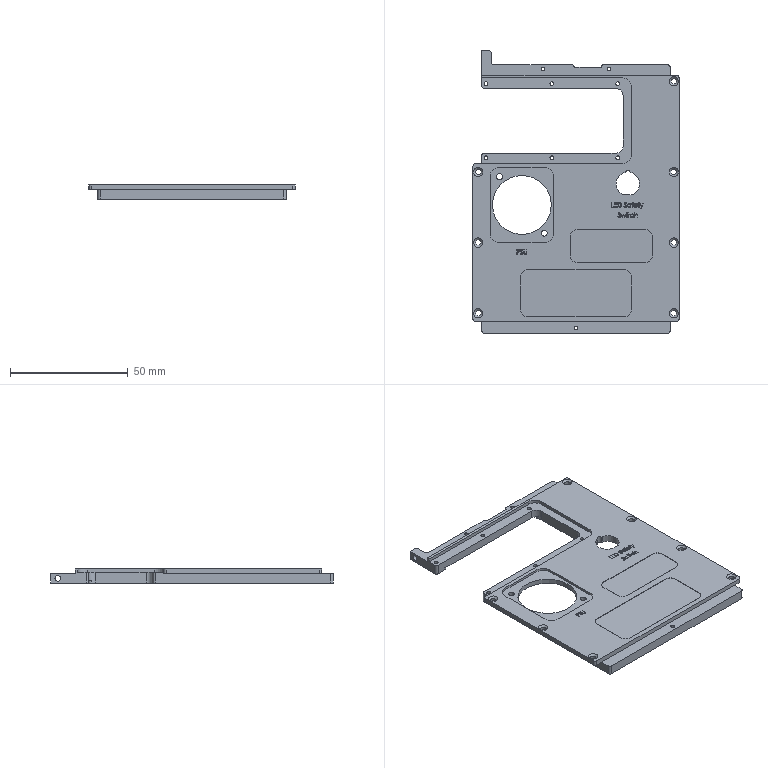NC program | NX | posted with a generic post | part box 87.5 x 120 x 6.001 mm
Whole program:
N10 G17 G21 G94 G90
(FLOOR_WALL_2 , TOOL : D63面刀)
N12 T01 M6
N14 G54
N16 G17 G0 G90 X96. Y-5. B0. C0. S4000 M3
N18 G43 Z50.001 H1
N20 Z6.545
N22 G94 G1 Z3.545 F1500.
N24 X86.
N26 X-97.
N28 Y41.55
N30 X86.
N32 X96.
N34 Z6.545
N36 G0 Z50.001
N38 Y-5.
N40 Z6.089
N42 G1 Z3.089
N44 X86.
N46 X-97.
N48 Y41.55
N50 X86.
N52 X96.
N54 Z6.089
N56 G0 Z50.001
N58 Y-5.
N60 Z5.632
N62 G1 Z2.632
N64 X86.
N66 X-97.
N68 Y41.55
N70 X86.
N72 X96.
N74 Z5.632
N76 G0 Z50.001
N78 Y-5.
N80 Z5.176
N82 G1 Z2.176
N84 X86.
N86 X-97.
N88 Y41.55
N90 X86.
N92 X96.
N94 Z5.176
N96 G0 Z50.001
N98 Y-5.
N100 Z4.72
N102 G1 Z1.72
N104 X86.
N106 X-97.
N108 Y41.55
N110 X86.
N112 X96.
N114 Z4.72
N116 G0 Z50.001
N118 Y-5.
N120 Z4.264
N122 G1 Z1.264
N124 X86.
N126 X-97.
N128 Y41.55
N130 X86.
N132 X96.
N134 Z4.264
N136 G0 Z50.001
N138 Y-5.
N140 Z3.807
N142 G1 Z0.807
N144 X86.
N146 X-97.
N148 Y41.55
N150 X86.
N152 X96.
N154 Z3.807
N156 G0 Z50.001
N158 Y-5.
N160 Z3.351
N162 G1 Z0.351
N164 X86.
N166 X-97.
N168 Y41.55
N170 X86.
N172 X96.
N174 Z3.351
N176 G0 Z50.001
N178 M5
(FLOOR_WALL_2_COPY , TOOL : D12-35-D12-75波刀)
N180 T13 M6
N182 G54
N184 G17 G0 G90 X70.5 Y-17.75 B0. C0. S4000 M3
N186 G43 Z50.001 H13
N188 Z3.031
N190 G94 G1 Z0.031 F1500.
N192 X60.5
N194 X-71.5
N196 Y-8.894
N198 X60.5
N200 Y-0.039
N202 X-71.5
N204 Y8.817
N206 X60.5
N208 Y17.672
N210 X-71.5
N212 Y26.528
N214 X60.5
N216 Y35.383
N218 X-71.5
N220 Y44.239
N222 X60.5
N224 Y53.094
N226 X-71.5
N228 Y61.95
N230 X60.5
N232 X70.5
N234 Z3.031
N236 G0 Z50.001
(FLOOR_WALL_2_COPY_COPY , TOOL : D12-35-D12-75波刀)
N238 Y-17.75 S5000
N240 Z3.001
N242 G1 Z0.001 F500.
N244 X60.5
N246 X-71.5
N248 Y-8.894
N250 X60.5
N252 Y-0.039
N254 X-71.5
N256 Y8.817
N258 X60.5
N260 Y17.672
N262 X-71.5
N264 Y26.528
N266 X60.5
N268 Y35.383
N270 X-71.5
N272 Y44.239
N274 X60.5
N276 Y53.094
N278 X-71.5
N280 Y61.95
N282 X60.5
N284 X70.5
N286 Z3.001
N288 G0 Z50.001
N290 M5
(PLANAR_MILL_5 , TOOL : D6-18-D6-50-3T-ROUGH)
N292 T02 M6
N294 G54
N296 G17 G0 G90 X0. Y-4.4 B0. C0. S5500 M3
N298 G43 Z50.001 H2
N300 Z2.5
N302 G94 G1 Z-0.5 F2500.
N304 Y-7.4
N306 X9.9
N308 Y7.4
N310 X-9.9
N312 Y-7.4
N314 X0.
N316 Y-4.4
N318 Y-10.4
N320 X12.
N322 G3 X12.9 Y-9.5 R0.9
N324 G1 Y9.5
N326 G3 X12. Y10.4 R0.9
N328 G1 X-12.
N330 G3 X-12.9 Y9.5 R0.9
N332 G1 Y-9.5
N334 G3 X-12. Y-10.4 R0.9
N336 G1 X0.
N338 Y-7.4
N340 Z2.5
N342 G0 Z50.001
N344 Y-4.4
N346 Z2.1
N348 G1 Z-0.9
N350 Y-7.4
N352 X9.9
N354 Y7.4
N356 X-9.9
N358 Y-7.4
N360 X0.
N362 Y-4.4
N364 Y-10.4
N366 X12.
N368 G3 X12.9 Y-9.5 R0.9
N370 G1 Y9.5
N372 G3 X12. Y10.4 R0.9
N374 G1 X-12.
N376 G3 X-12.9 Y9.5 R0.9
N378 G1 Y-9.5
N380 G3 X-12. Y-10.4 R0.9
N382 G1 X0.
N384 Y-7.4
N386 Z2.1
N388 G0 Z50.001
(PLANAR_MILL_5_COPY_2 , TOOL : D6-18-D6-50-3T-ROUGH)
N390 X-20.6 Y-25.75
N392 Z2.5
N394 G1 Z-0.5
N396 Y-19.75
N398 Y42.5
N400 G3 X-21.5 Y43.4 R0.9
N402 G1 X-50.
N404 G3 X-50.9 Y42.5 R0.9
N406 G1 Y-17.
N408 Y-23.
N410 Z2.5
N412 G0 X-20.6 Y-25.75 Z2.
N414 G1 Z-1.
N416 Y-19.75
N418 Y42.5
N420 G3 X-21.5 Y43.4 R0.9
N422 G1 X-50.
N424 G3 X-50.9 Y42.5 R0.9
N426 G1 Y-17.
N428 Y-23.
N430 Z2.
N432 G0 X-20.6 Y-25.75 Z1.6
N434 G1 Z-1.4
N436 Y-19.75
N438 Y42.5
N440 G3 X-21.5 Y43.4 R0.9
N442 G1 X-50.
N444 G3 X-50.9 Y42.5 R0.9
N446 G1 Y-17.
N448 Y-23.
N450 Z1.6
N452 G0 Z50.001
N454 M5
(PLANAR_MILL_5_COPY , TOOL : D6-18-D6-50-3T-FINISH)
N456 T05 M6
N458 G54
N460 G17 G0 G90 X17.458 Y49. B0. C0. S5464 M3
N462 G43 Z50.001 H5
N464 Z0.
N466 G94 G1 X17. Z-0.008 F500.
N468 Y38. Z-0.2
N470 X16.5
N472 Y26.5
N474 X18.5
N476 Y49.5
N478 X16.5
N480 Y38.
N482 Z0.
N484 G0 X14. Y49.458
N486 G1 Y38. Z-0.2
N488 X13.5
N490 Y23.5
N492 X21.5
N494 Y52.5
N496 X13.5
N498 Y38.
N500 X14.025 Z0.325
N502 G0 Z50.001
N504 X39.8 Y11.542
N506 Z0.
N508 G1 Y23. Z-0.2
N510 X40.3
N512 Y39.3
N514 X34.7
N516 Y6.7
N518 X40.3
N520 Y23.
N522 Z0.
N524 G0 X44. Y11.542
N526 G1 Y23. Z-0.2
N528 X44.5
N530 Y43.5
N532 X30.5
N534 Y2.5
N536 X44.5
N538 Y23.
N540 X43.975 Z0.325
N542 G0 Z50.001
(PLANAR_MILL_5_COPY_1 , TOOL : D6-18-D6-50-3T-FINISH)
N544 X-0.5 Y-7.
N546 Z2.
N548 G1 Z-1.
N550 G3 X0. Y-7.5 R0.5
N552 G1 X10.
N554 Y7.5
N556 X-10.
N558 Y-7.5
N560 X0.
N562 G3 X0.5 Y-7. R0.5
N564 G1 X-0.5 Y-10.
N566 G3 X0. Y-10.5 R0.5
N568 G1 X12.
N570 G3 X13. Y-9.5 R1.
N572 G1 Y9.5
N574 G3 X12. Y10.5 R1.
N576 G1 X-12.
N578 G3 X-13. Y9.5 R1.
N580 G1 Y-9.5
N582 G3 X-12. Y-10.5 R1.
N584 G1 X0.
N586 G3 X0.5 Y-10. R0.5
N588 G1 Z2.
N590 G0 Z50.001
(PLANAR_MILL_5_COPY_2_COPY , TOOL : D6-18-D6-50-3T-FINISH)
N592 X-20.5 Y-25.75
N594 Z1.5
N596 G1 Z-1.5
N598 Y-19.75
N600 Y42.5
N602 G3 X-21.5 Y43.5 R1.
N604 G1 X-50.
N606 G3 X-51. Y42.5 R1.
N608 G1 Y-17.
N610 Y-23.
N612 Z1.5
N614 G0 Z50.001
N616 M5
(PLANAR_MILL_4 , TOOL : D12-35-D12-75波刀)
N618 T13 M6
N620 G54
N622 G17 G0 G90 X55.6 Y77.75 B0. C0. S5500 M3
N624 G43 Z50.001 H13
N626 Z2.
N628 G94 G1 Z-1. F2500.
N630 Y65.75
N632 Y-19.75
N634 Y-31.75
N636 Z2.
N638 G0 Z3.
N640 Y77.75
N642 Z1.1
N644 G1 Z-1.9
N646 Y65.75
N648 Y-19.75
N650 Y-31.75
N652 Z1.1
N654 G0 Z50.001
(PLANAR_MILL_4_COPY , TOOL : D12-35-D12-75波刀)
N656 X-61.1 Y-29.
N658 Z2.
N660 G1 Z-1.
N662 Y-17.
N664 Y65.75
N666 Y77.75
N668 Z2.
N670 G0 Z3.
N672 Y-29.
N674 Z1.1
N676 G1 Z-1.9
N678 Y-17.
N680 Y65.75
N682 Y77.75
N684 Z1.1
N686 G0 Z50.001
N688 M5
(PLANAR_MILL_4_COPY_COPY , TOOL : D6-18-D6-50-3T-FINISH)
N690 T05 M6
N692 G54
N694 G17 G0 G90 X-63.5 Y-8. B0. C0. S5500 M3
N696 G43 Z50.001 H5
N698 Z1.
N700 G94 G1 Z-2. F2500.
N702 Y-14.
N704 Y-17.
N706 Y-23.
N708 Z1.
N710 G0 Z50.001
(PLANAR_MILL_4_COPY_COPY_COPY , TOOL : D6-18-D6-50-3T-FINISH)
N712 X-59. Y-18.
N714 Z1.
N716 G1 Z-2.
N718 G3 X-58. Y-17. R1.
N720 G1 Y65.75
N722 G2 X-54. Y69.75 R4.
N724 G1 X48.5
N726 G2 X52.5 Y65.75 R4.
N728 G1 Y-19.75
N730 G2 X48.5 Y-23.75 R4.
N732 G1 X-16.5
N734 G3 X-17.5 Y-24.75 R1.
N736 G1 Z1.
N738 G0 Z50.001
N740 M5
(SPOT_DRILLING_2 , TOOL : 点孔D5-120-90度)
N742 T14 M6
N744 G54
N746 G17 G0 G90 X-14. Y-18.5 B0. C0. S2500 M3
N748 G43 Z50.001 H14
N750 G94 G82 G99 Z-2. F120. P200 R2.
N752 X16.
N754 X46.
N756 Y64.5
N758 X16.
N760 X-14.
N762 X-52.5
N764 G80
N766 G0 X-52.5 Y64.5 Z50.001
(SPOT_DRILLING_2_COPY , TOOL : 点孔D5-120-90度)
N768 X-12. Y-9.5
N770 G82 Z-2.25 F120. P200 R1.
N772 X12. Y9.5
N774 G80
N776 G0 X12. Y9.5 Z50.001
N778 M5
(SPOT_DRILLING_2_COPY_COPY , TOOL : 点孔D3-50-90度)
N780 T07 M6
N782 G54
N784 G17 G0 G90 X52.25 Y23. B0. C0. S2500 M3
N786 G43 Z10. H7
N788 G94 G82 G98 Z-3.02 F120. P200 R0.
N790 X-20. Y40.75 Z-2.52 R0.5
N792 Y12.75
N794 Y-15.25
N796 X-51.5
N798 X-57.75 Y9. Z-3.02 R0.
N800 X-51.5 Y12.75 Z-2.52 R0.5
N802 X-57.75 Y37. Z-3.02 R0.
N804 X-51.5 Y40.75 Z-2.52 R0.5
N806 G80
N808 G0 X-51.5 Y40.75 Z10.
(PLANAR_MILL_7 , TOOL : 点孔D3-50-90度)
N810 Z50.001 S6500
N812 X-2.75 Y69.05
N814 Z2.2
N816 G1 Z-0.8 F1500.
N818 Y67.55
N820 X48.5
N822 G2 X50.3 Y65.75 R1.8
N824 G1 Y-19.75
N826 G2 X48.5 Y-21.55 R1.8
N828 G1 X-16.5
N830 G2 X-18.3 Y-19.75 R1.8
N832 G1 Y42.5
N834 G3 X-21.5 Y45.7 R3.2
N836 G1 X-50.
N838 G3 X-53.2 Y42.5 R3.2
N840 G1 Y-17.
N842 G2 X-54. Y-17.8 R0.8
N844 G1 X-55.
N846 G2 X-55.8 Y-17. R0.8
N848 G1 Y65.75
N850 G2 X-54. Y67.55 R1.8
N852 G1 X-2.75
N854 Y69.05
N856 Z2.2
N858 G0 Z50.001
(PLANAR_MILL_7_COPY_1 , TOOL : 点孔D3-50-90度)
N860 X-20.5 Y-18.3
N862 Z0.7
N864 G1 Z-2.3
N866 G3 X-21. Y-17.8 R0.5
N868 G2 X-22.8 Y-16. R1.8
N870 G1 Y40.
N872 G3 X-25. Y42.2 R2.2
N874 G1 X-46.5
N876 G3 X-48.7 Y40. R2.2
N878 G1 Y-16.
N880 G2 X-50.5 Y-17.8 R1.8
N882 G3 X-51. Y-18.3 R0.5
N884 G1 Z0.7
N886 G0 Z50.001
(PLANAR_MILL_7_COPY , TOOL : 点孔D3-50-90度)
N888 X0. Y-11.2
N890 Z2.2
N892 G1 Z-0.8
N894 Y-12.7
N896 X12.
N898 G3 X15.2 Y-9.5 R3.2
N900 G1 Y9.5
N902 G3 X12. Y12.7 R3.2
N904 G1 X-12.
N906 G3 X-15.2 Y9.5 R3.2
N908 G1 Y-9.5
N910 G3 X-12. Y-12.7 R3.2
N912 G1 X0.
N914 Y-11.2
N916 Z2.2
N918 G0 Z50.001
N920 X-6.65 Y45.
N922 Z2.2
N924 G1 Z-0.8
N926 X-5.15
N928 Y46.679
N930 G3 X-12.85 Y46.679 R4.2
N932 G1 Y46.
N934 G2 X-13.65 Y45.2 R0.8
N936 G3 X-13.85 Y45. R0.2
N938 X-13.65 Y44.8 R0.2
N940 G2 X-12.85 Y44. R0.8
N942 G1 Y43.321
N944 G3 X-5.15 Y43.321 R4.2
N946 G1 Y45.
N948 X-6.65
N950 Z2.2
N952 G0 Z50.001
(PLANAR_MILL_7_COPY_COPY , TOOL : 点孔D3-50-90度)
N954 X53.2 Y64.1
N956 Z0.2
N958 G1 Z-2.8
N960 G3 X53.5 Y63.8 R0.3
N962 G2 X55.3 Y62. R1.8
N964 G1 Y-16.
N966 G2 X53.5 Y-17.8 R1.8
N968 G3 X53.2 Y-18.1 R0.3
N970 G1 Z0.2
N972 G0 Z50.001
N974 X-57.
N976 Z0.2
N978 G1 Z-2.8
N980 G3 X-57.3 Y-17.8 R0.3
N982 G1 X-65.5
N984 G2 X-66.3 Y-17. R0.8
N986 G1 Y-14.
N988 G2 X-64.5 Y-12.2 R1.8
N990 G1 X-60.5
N992 G3 X-60.3 Y-12. R0.2
N994 G1 Y21.5
N996 G2 X-59.3 Y22.765 R1.3
N998 G1 Y33.235
N1000 G2 X-60.3 Y34.5 R1.3
N1002 G1 Y62.
N1004 G2 X-58.5 Y63.8 R1.8
N1006 G3 X-58.2 Y64.1 R0.3
N1008 G1 Z0.2
N1010 G0 Z50.001
N1012 M5
(PLANAR_MILL_COPY_COPY_COPY_COPY_COPY_COPY_COPY_1 , TOOL : D2-6-D4-50-3T-FINISH)
N1014 T04 M6
N1016 G54
N1018 G17 G0 G90 X-16.474 Y-22.965 B0. C0. S5500 M3
N1020 G43 Z50.001 H4
N1022 Z0.9
N1024 G94 G1 Z-2.1 F400.
N1026 G41 X-16.3 Y-21.98 D4
N1028 G3 X-16.5 Y-21.78 R0.2
N1030 G2 X-18.53 Y-19.75 R2.03
N1032 G3 X-18.73 Y-19.55 R0.2
N1034 G40
N1036 G1 X-19.715 Y-19.724
N1038 Z0.9
N1040 G0 Z50.001
N1042 M5
(SPOT_DRILLING_2_COPY_1 , TOOL : Z2.4)
N1044 T15 M6
N1046 G54
N1048 G17 G0 G90 X-14. Y-18.5 B0. C0. S2500 M3
N1050 G43 Z10. H15
N1052 G94 G82 G98 Z-5. F120. P200 R2.
N1054 X16.
N1056 X46.
N1058 Y64.5
N1060 X16.
N1062 X-14.
N1064 X-52.5
N1066 G80
N1068 G0 X-52.5 Y64.5 Z10.
N1070 M5
N1072 M2